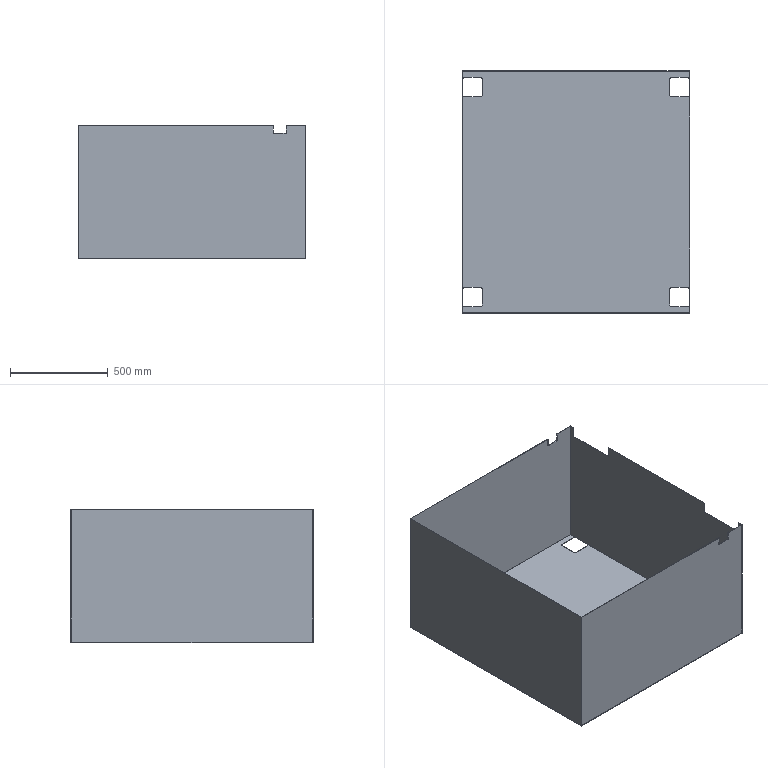Part | SolidWorks | features BaseBody 1 | 1 solid | 54 faces | box 1164 x 1240 x 681 mm | volume 9260336 mm3 | plane 38 | cylinder 16 | commonest cylinder face diameters 20 x16